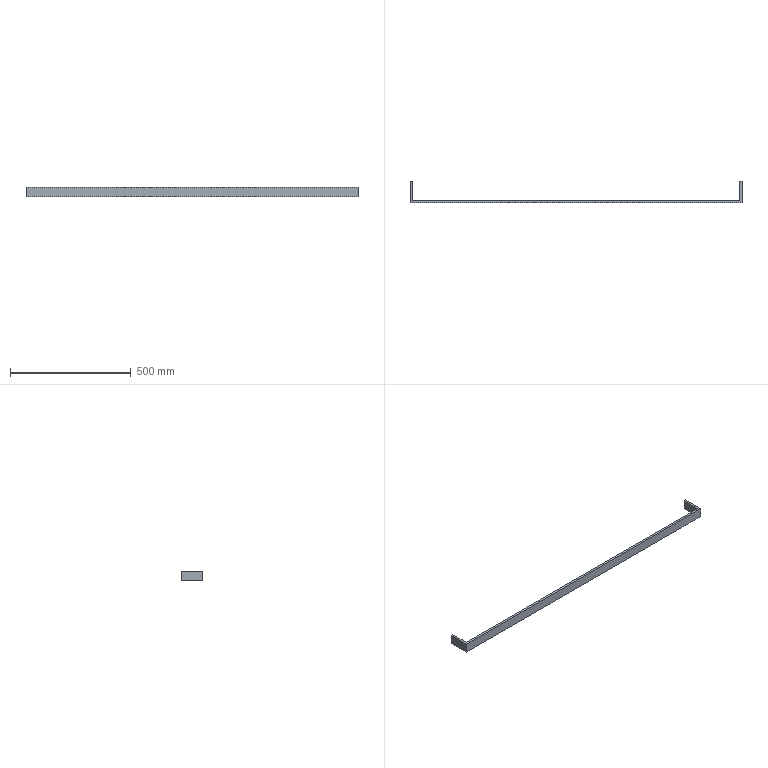Part | SolidWorks | features Extrusion 1, ICE 1, MirrorPattern 1 | 1 solid | 10 faces | box 1374 x 89 x 40 mm | volume 612800 mm3 | plane 10
STEP:
#1=CARTESIAN_POINT('',(687.,0.,-20.));
#2=VERTEX_POINT('',#1);
#3=CARTESIAN_POINT('',(-687.,0.,-20.));
#4=VERTEX_POINT('',#3);
#5=CARTESIAN_POINT('',(-677.,0.,-20.));
#6=DIRECTION('',(-1.,0.,0.));
#7=VECTOR('',#6,1000.);
#8=LINE('',#5,#7);
#9=EDGE_CURVE('',#2,#4,#8,.T.);
#10=ORIENTED_EDGE('',*,*,#9,.T.);
#11=CARTESIAN_POINT('',(-687.,89.,-20.));
#12=VERTEX_POINT('',#11);
#13=CARTESIAN_POINT('',(-687.,0.,-20.));
#14=DIRECTION('',(0.,-1.,0.));
#15=VECTOR('',#14,1000.);
#16=LINE('',#13,#15);
#17=EDGE_CURVE('',#12,#4,#16,.T.);
#18=ORIENTED_EDGE('',*,*,#17,.F.);
#19=CARTESIAN_POINT('',(-677.,89.,-20.));
#20=VERTEX_POINT('',#19);
#21=CARTESIAN_POINT('',(-687.,89.,-20.));
#22=DIRECTION('',(1.,0.,0.));
#23=VECTOR('',#22,1000.);
#24=LINE('',#21,#23);
#25=EDGE_CURVE('',#12,#20,#24,.T.);
#26=ORIENTED_EDGE('',*,*,#25,.T.);
#27=CARTESIAN_POINT('',(-677.,10.,-20.));
#28=VERTEX_POINT('',#27);
#29=CARTESIAN_POINT('',(-677.,0.,-20.));
#30=DIRECTION('',(0.,-1.,0.));
#31=VECTOR('',#30,1000.);
#32=LINE('',#29,#31);
#33=EDGE_CURVE('',#20,#28,#32,.T.);
#34=ORIENTED_EDGE('',*,*,#33,.T.);
#35=CARTESIAN_POINT('',(677.,10.,-20.));
#36=VERTEX_POINT('',#35);
#37=CARTESIAN_POINT('',(-677.,10.,-20.));
#38=DIRECTION('',(-1.,0.,0.));
#39=VECTOR('',#38,1000.);
#40=LINE('',#37,#39);
#41=EDGE_CURVE('',#36,#28,#40,.T.);
#42=ORIENTED_EDGE('',*,*,#41,.F.);
#43=CARTESIAN_POINT('',(677.,89.,-20.));
#44=VERTEX_POINT('',#43);
#45=CARTESIAN_POINT('',(677.,0.,-20.));
#46=DIRECTION('',(0.,-1.,0.));
#47=VECTOR('',#46,1000.);
#48=LINE('',#45,#47);
#49=EDGE_CURVE('',#44,#36,#48,.T.);
#50=ORIENTED_EDGE('',*,*,#49,.F.);
#51=CARTESIAN_POINT('',(687.,89.,-20.));
#52=VERTEX_POINT('',#51);
#53=CARTESIAN_POINT('',(687.,89.,-20.));
#54=DIRECTION('',(-1.,0.,0.));
#55=VECTOR('',#54,1000.);
#56=LINE('',#53,#55);
#57=EDGE_CURVE('',#52,#44,#56,.T.);
#58=ORIENTED_EDGE('',*,*,#57,.F.);
#59=CARTESIAN_POINT('',(687.,0.,-20.));
#60=DIRECTION('',(0.,-1.,0.));
#61=VECTOR('',#60,1000.);
#62=LINE('',#59,#61);
#63=EDGE_CURVE('',#52,#2,#62,.T.);
#64=ORIENTED_EDGE('',*,*,#63,.T.);
#65=EDGE_LOOP('',(#10,#18,#26,#34,#42,#50,#58,#64));
#66=FACE_OUTER_BOUND('',#65,.T.);
#67=CARTESIAN_POINT('',(-677.,10.,-20.));
#68=DIRECTION('',(0.,0.,1.));
#69=DIRECTION('',(1.,0.,0.));
#70=AXIS2_PLACEMENT_3D('',#67,#68,#69);
#71=PLANE('',#70);
#72=ADVANCED_FACE('',(#66),#71,.F.);
#73=CARTESIAN_POINT('',(-687.,0.,20.));
#74=VERTEX_POINT('',#73);
#75=CARTESIAN_POINT('',(687.,0.,20.));
#76=VERTEX_POINT('',#75);
#77=CARTESIAN_POINT('',(-677.,0.,20.));
#78=DIRECTION('',(1.,0.,0.));
#79=VECTOR('',#78,1000.);
#80=LINE('',#77,#79);
#81=EDGE_CURVE('',#74,#76,#80,.T.);
#82=ORIENTED_EDGE('',*,*,#81,.T.);
#83=CARTESIAN_POINT('',(687.,89.,20.));
#84=VERTEX_POINT('',#83);
#85=CARTESIAN_POINT('',(687.,0.,20.));
#86=DIRECTION('',(0.,1.,0.));
#87=VECTOR('',#86,1000.);
#88=LINE('',#85,#87);
#89=EDGE_CURVE('',#76,#84,#88,.T.);
#90=ORIENTED_EDGE('',*,*,#89,.T.);
#91=CARTESIAN_POINT('',(677.,89.,20.));
#92=VERTEX_POINT('',#91);
#93=CARTESIAN_POINT('',(687.,89.,20.));
#94=DIRECTION('',(-1.,0.,0.));
#95=VECTOR('',#94,1000.);
#96=LINE('',#93,#95);
#97=EDGE_CURVE('',#84,#92,#96,.T.);
#98=ORIENTED_EDGE('',*,*,#97,.T.);
#99=CARTESIAN_POINT('',(677.,10.,20.));
#100=VERTEX_POINT('',#99);
#101=CARTESIAN_POINT('',(677.,0.,20.));
#102=DIRECTION('',(0.,1.,0.));
#103=VECTOR('',#102,1000.);
#104=LINE('',#101,#103);
#105=EDGE_CURVE('',#100,#92,#104,.T.);
#106=ORIENTED_EDGE('',*,*,#105,.F.);
#107=CARTESIAN_POINT('',(-677.,10.,20.));
#108=VERTEX_POINT('',#107);
#109=CARTESIAN_POINT('',(-677.,10.,20.));
#110=DIRECTION('',(1.,0.,0.));
#111=VECTOR('',#110,1000.);
#112=LINE('',#109,#111);
#113=EDGE_CURVE('',#108,#100,#112,.T.);
#114=ORIENTED_EDGE('',*,*,#113,.F.);
#115=CARTESIAN_POINT('',(-677.,89.,20.));
#116=VERTEX_POINT('',#115);
#117=CARTESIAN_POINT('',(-677.,0.,20.));
#118=DIRECTION('',(0.,1.,0.));
#119=VECTOR('',#118,1000.);
#120=LINE('',#117,#119);
#121=EDGE_CURVE('',#108,#116,#120,.T.);
#122=ORIENTED_EDGE('',*,*,#121,.T.);
#123=CARTESIAN_POINT('',(-687.,89.,20.));
#124=VERTEX_POINT('',#123);
#125=CARTESIAN_POINT('',(-687.,89.,20.));
#126=DIRECTION('',(1.,0.,0.));
#127=VECTOR('',#126,1000.);
#128=LINE('',#125,#127);
#129=EDGE_CURVE('',#124,#116,#128,.T.);
#130=ORIENTED_EDGE('',*,*,#129,.F.);
#131=CARTESIAN_POINT('',(-687.,0.,20.));
#132=DIRECTION('',(0.,1.,0.));
#133=VECTOR('',#132,1000.);
#134=LINE('',#131,#133);
#135=EDGE_CURVE('',#74,#124,#134,.T.);
#136=ORIENTED_EDGE('',*,*,#135,.F.);
#137=EDGE_LOOP('',(#82,#90,#98,#106,#114,#122,#130,#136));
#138=FACE_OUTER_BOUND('',#137,.T.);
#139=CARTESIAN_POINT('',(-677.,10.,20.));
#140=DIRECTION('',(0.,0.,-1.));
#141=DIRECTION('',(-1.,0.,0.));
#142=AXIS2_PLACEMENT_3D('',#139,#140,#141);
#143=PLANE('',#142);
#144=ADVANCED_FACE('',(#138),#143,.F.);
#145=CARTESIAN_POINT('',(677.,10.,-20.));
#146=DIRECTION('',(0.,0.,-1.));
#147=VECTOR('',#146,1000.);
#148=LINE('',#145,#147);
#149=EDGE_CURVE('',#100,#36,#148,.T.);
#150=ORIENTED_EDGE('',*,*,#149,.T.);
#151=ORIENTED_EDGE('',*,*,#41,.T.);
#152=CARTESIAN_POINT('',(-677.,10.,-20.));
#153=DIRECTION('',(0.,0.,1.));
#154=VECTOR('',#153,1000.);
#155=LINE('',#152,#154);
#156=EDGE_CURVE('',#28,#108,#155,.T.);
#157=ORIENTED_EDGE('',*,*,#156,.T.);
#158=ORIENTED_EDGE('',*,*,#113,.T.);
#159=EDGE_LOOP('',(#150,#151,#157,#158));
#160=FACE_OUTER_BOUND('',#159,.T.);
#161=CARTESIAN_POINT('',(0.,10.,0.));
#162=DIRECTION('',(0.,1.,0.));
#163=DIRECTION('',(0.,0.,1.));
#164=AXIS2_PLACEMENT_3D('',#161,#162,#163);
#165=PLANE('',#164);
#166=ADVANCED_FACE('',(#160),#165,.T.);
#167=ORIENTED_EDGE('',*,*,#9,.F.);
#168=CARTESIAN_POINT('',(687.,0.,-20.));
#169=DIRECTION('',(0.,0.,1.));
#170=VECTOR('',#169,1000.);
#171=LINE('',#168,#170);
#172=EDGE_CURVE('',#2,#76,#171,.T.);
#173=ORIENTED_EDGE('',*,*,#172,.T.);
#174=ORIENTED_EDGE('',*,*,#81,.F.);
#175=CARTESIAN_POINT('',(-687.,0.,-20.));
#176=DIRECTION('',(0.,0.,1.));
#177=VECTOR('',#176,1000.);
#178=LINE('',#175,#177);
#179=EDGE_CURVE('',#4,#74,#178,.T.);
#180=ORIENTED_EDGE('',*,*,#179,.F.);
#181=EDGE_LOOP('',(#167,#173,#174,#180));
#182=FACE_OUTER_BOUND('',#181,.T.);
#183=CARTESIAN_POINT('',(0.,0.,0.));
#184=DIRECTION('',(0.,1.,0.));
#185=DIRECTION('',(0.,0.,1.));
#186=AXIS2_PLACEMENT_3D('',#183,#184,#185);
#187=PLANE('',#186);
#188=ADVANCED_FACE('',(#182),#187,.F.);
#189=ORIENTED_EDGE('',*,*,#156,.F.);
#190=ORIENTED_EDGE('',*,*,#33,.F.);
#191=CARTESIAN_POINT('',(-677.,89.,-20.));
#192=DIRECTION('',(0.,0.,-1.));
#193=VECTOR('',#192,1000.);
#194=LINE('',#191,#193);
#195=EDGE_CURVE('',#116,#20,#194,.T.);
#196=ORIENTED_EDGE('',*,*,#195,.F.);
#197=ORIENTED_EDGE('',*,*,#121,.F.);
#198=EDGE_LOOP('',(#189,#190,#196,#197));
#199=FACE_OUTER_BOUND('',#198,.T.);
#200=CARTESIAN_POINT('',(-677.,0.,0.));
#201=DIRECTION('',(1.,0.,0.));
#202=DIRECTION('',(0.,0.,-1.));
#203=AXIS2_PLACEMENT_3D('',#200,#201,#202);
#204=PLANE('',#203);
#205=ADVANCED_FACE('',(#199),#204,.T.);
#206=ORIENTED_EDGE('',*,*,#195,.T.);
#207=ORIENTED_EDGE('',*,*,#25,.F.);
#208=CARTESIAN_POINT('',(-687.,89.,-20.));
#209=DIRECTION('',(0.,0.,-1.));
#210=VECTOR('',#209,1000.);
#211=LINE('',#208,#210);
#212=EDGE_CURVE('',#124,#12,#211,.T.);
#213=ORIENTED_EDGE('',*,*,#212,.F.);
#214=ORIENTED_EDGE('',*,*,#129,.T.);
#215=EDGE_LOOP('',(#206,#207,#213,#214));
#216=FACE_OUTER_BOUND('',#215,.T.);
#217=CARTESIAN_POINT('',(-687.,89.,-20.));
#218=DIRECTION('',(0.,-1.,0.));
#219=DIRECTION('',(0.,0.,-1.));
#220=AXIS2_PLACEMENT_3D('',#217,#218,#219);
#221=PLANE('',#220);
#222=ADVANCED_FACE('',(#216),#221,.F.);
#223=ORIENTED_EDGE('',*,*,#17,.T.);
#224=ORIENTED_EDGE('',*,*,#179,.T.);
#225=ORIENTED_EDGE('',*,*,#135,.T.);
#226=ORIENTED_EDGE('',*,*,#212,.T.);
#227=EDGE_LOOP('',(#223,#224,#225,#226));
#228=FACE_OUTER_BOUND('',#227,.T.);
#229=CARTESIAN_POINT('',(-687.,0.,0.));
#230=DIRECTION('',(1.,0.,0.));
#231=DIRECTION('',(0.,0.,-1.));
#232=AXIS2_PLACEMENT_3D('',#229,#230,#231);
#233=PLANE('',#232);
#234=ADVANCED_FACE('',(#228),#233,.F.);
#235=ORIENTED_EDGE('',*,*,#149,.F.);
#236=ORIENTED_EDGE('',*,*,#105,.T.);
#237=CARTESIAN_POINT('',(677.,89.,-20.));
#238=DIRECTION('',(0.,0.,-1.));
#239=VECTOR('',#238,1000.);
#240=LINE('',#237,#239);
#241=EDGE_CURVE('',#92,#44,#240,.T.);
#242=ORIENTED_EDGE('',*,*,#241,.T.);
#243=ORIENTED_EDGE('',*,*,#49,.T.);
#244=EDGE_LOOP('',(#235,#236,#242,#243));
#245=FACE_OUTER_BOUND('',#244,.T.);
#246=CARTESIAN_POINT('',(677.,0.,0.));
#247=DIRECTION('',(-1.,0.,0.));
#248=DIRECTION('',(0.,0.,-1.));
#249=AXIS2_PLACEMENT_3D('',#246,#247,#248);
#250=PLANE('',#249);
#251=ADVANCED_FACE('',(#245),#250,.T.);
#252=ORIENTED_EDGE('',*,*,#241,.F.);
#253=ORIENTED_EDGE('',*,*,#97,.F.);
#254=CARTESIAN_POINT('',(687.,89.,-20.));
#255=DIRECTION('',(0.,0.,-1.));
#256=VECTOR('',#255,1000.);
#257=LINE('',#254,#256);
#258=EDGE_CURVE('',#84,#52,#257,.T.);
#259=ORIENTED_EDGE('',*,*,#258,.T.);
#260=ORIENTED_EDGE('',*,*,#57,.T.);
#261=EDGE_LOOP('',(#252,#253,#259,#260));
#262=FACE_OUTER_BOUND('',#261,.T.);
#263=CARTESIAN_POINT('',(687.,89.,-20.));
#264=DIRECTION('',(0.,1.,0.));
#265=DIRECTION('',(0.,0.,1.));
#266=AXIS2_PLACEMENT_3D('',#263,#264,#265);
#267=PLANE('',#266);
#268=ADVANCED_FACE('',(#262),#267,.T.);
#269=ORIENTED_EDGE('',*,*,#63,.F.);
#270=ORIENTED_EDGE('',*,*,#258,.F.);
#271=ORIENTED_EDGE('',*,*,#89,.F.);
#272=ORIENTED_EDGE('',*,*,#172,.F.);
#273=EDGE_LOOP('',(#269,#270,#271,#272));
#274=FACE_OUTER_BOUND('',#273,.T.);
#275=CARTESIAN_POINT('',(687.,0.,0.));
#276=DIRECTION('',(-1.,0.,0.));
#277=DIRECTION('',(0.,0.,-1.));
#278=AXIS2_PLACEMENT_3D('',#275,#276,#277);
#279=PLANE('',#278);
#280=ADVANCED_FACE('',(#274),#279,.F.);
#281=CLOSED_SHELL('',(#72,#144,#166,#188,#205,#222,#234,#251,#268,#280));
#282=MANIFOLD_SOLID_BREP('',#281);
#283=CARTESIAN_POINT('',(0.,0.,0.));
#284=DIRECTION('',(0.,0.,1.));
#285=DIRECTION('',(1.,0.,0.));
#286=AXIS2_PLACEMENT_3D('',#283,#284,#285);
#287=(LENGTH_UNIT()NAMED_UNIT(*)SI_UNIT(.MILLI.,.METRE.));
#288=UNCERTAINTY_MEASURE_WITH_UNIT(LENGTH_MEASURE(0.00001),#287,'','');
#289=(NAMED_UNIT(*)PLANE_ANGLE_UNIT()SI_UNIT($,.RADIAN.));
#290=(NAMED_UNIT(*)SI_UNIT($,.STERADIAN.)SOLID_ANGLE_UNIT());
#291=(GEOMETRIC_REPRESENTATION_CONTEXT(3)GLOBAL_UNCERTAINTY_ASSIGNED_CONTEXT((#288))GLOBAL_UNIT_ASSIGNED_CONTEXT((#287,#289,#290))REPRESENTATION_CONTEXT('',''));
#292=ADVANCED_BREP_SHAPE_REPRESENTATION('',(#282,#286),#291);